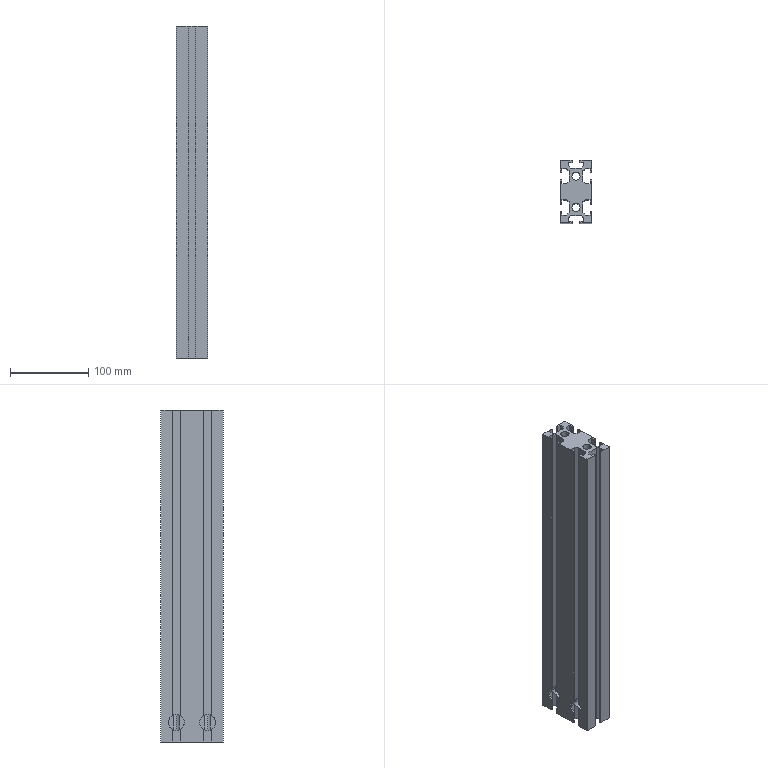Part | SolidWorks | features BaseBody 1 | 1 solid | 96 faces | box 40 x 80 x 425 mm | volume 813659 mm3 | plane 88 | cylinder 8 | commonest cylinder face diameters 10.5 x4 20.5 x4